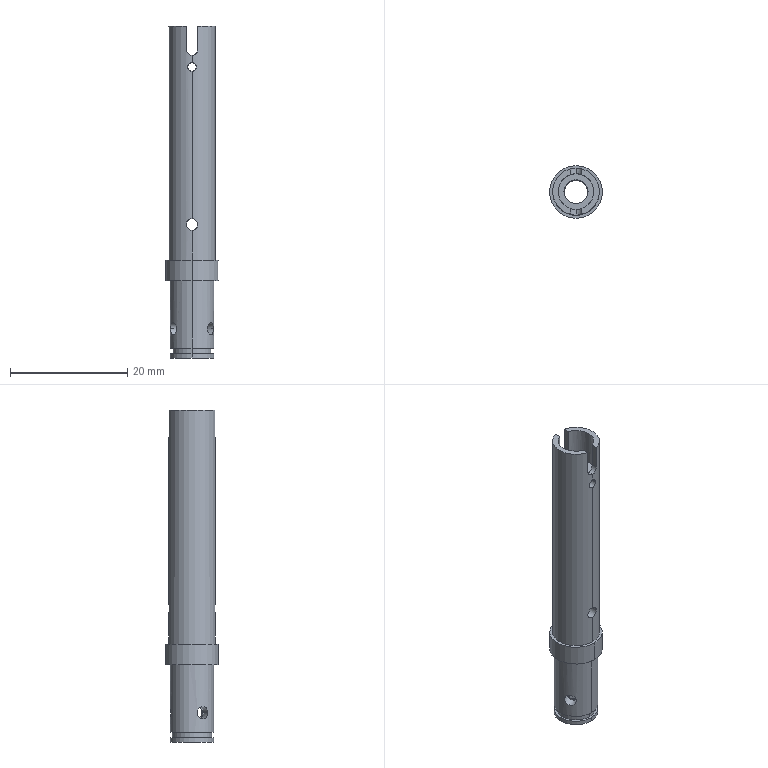Part | STEP file | ASND-0110-4216111600 | 1 solid | 56 faces | box 9 x 9 x 56.7 mm | volume 1924 mm3 | cylinder 40 | plane 16 | commonest cylinder face diameters 2 x8 1.8 x6 2.1 x6 1.5 x4 7.5 x4 4 x2